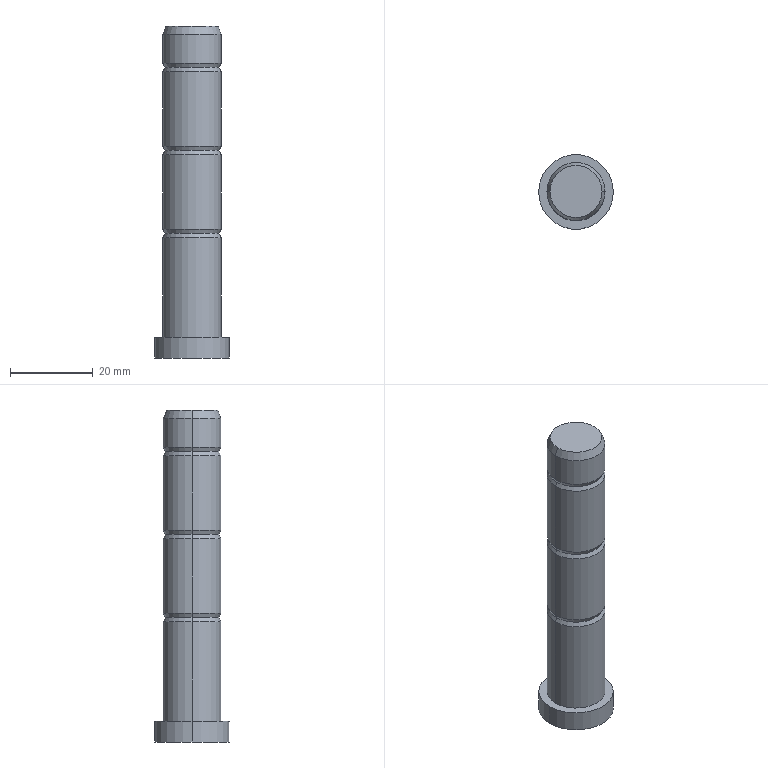Part | STEP file | EES - 2C 12x100 | 1 solid | 27 faces | box 18 x 18 x 80 mm | volume 12722 mm3 | cone 14 | cylinder 10 | plane 3 | commonest cylinder face diameters 14 x8 18 x2